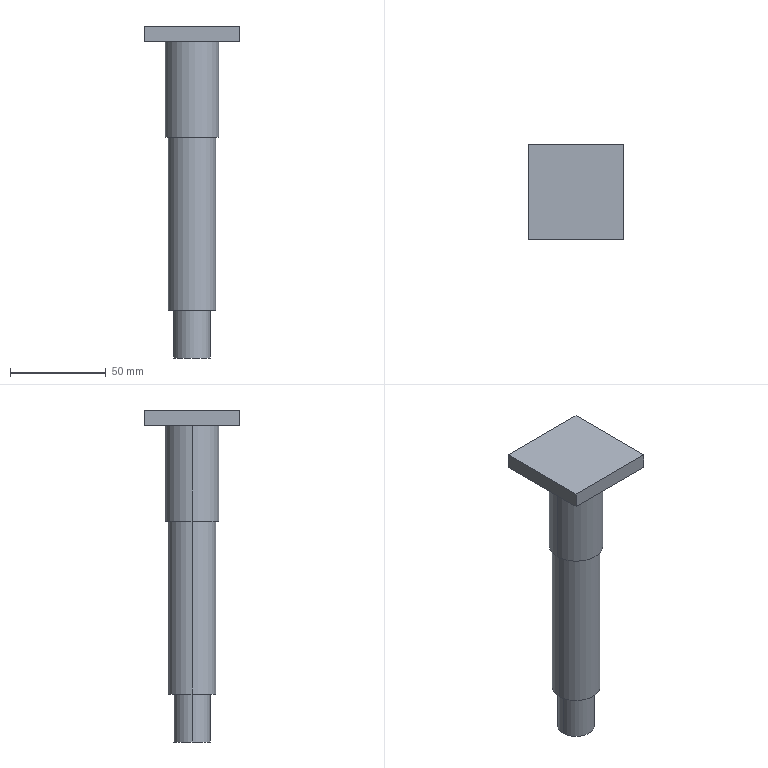Part | SolidWorks | features ICE 3, Extrusion 1 | 1 solid | 15 faces | box 50 x 50 x 173 mm | volume 102054 mm3 | plane 9 | cylinder 6 | commonest cylinder face diameters 19 x2 25 x2 28 x2
STEP:
#1=CARTESIAN_POINT('',(-9.5,0.,-25.));
#2=VERTEX_POINT('',#1);
#3=CARTESIAN_POINT('',(9.5,0.,-25.));
#4=VERTEX_POINT('',#3);
#5=CARTESIAN_POINT('',(0.,0.,-25.));
#6=DIRECTION('',(0.,0.,-1.));
#7=DIRECTION('',(-1.,0.,0.));
#8=AXIS2_PLACEMENT_3D('',#5,#6,#7);
#9=CIRCLE('',#8,9.5);
#10=EDGE_CURVE('',#2,#4,#9,.T.);
#11=ORIENTED_EDGE('',*,*,#10,.F.);
#12=CARTESIAN_POINT('',(-9.5,0.,0.));
#13=VERTEX_POINT('',#12);
#14=CARTESIAN_POINT('',(-9.5,0.,-25.));
#15=DIRECTION('',(0.,0.,1.));
#16=VECTOR('',#15,1000.);
#17=LINE('',#14,#16);
#18=EDGE_CURVE('',#2,#13,#17,.T.);
#19=ORIENTED_EDGE('',*,*,#18,.T.);
#20=CARTESIAN_POINT('',(9.5,0.,0.));
#21=VERTEX_POINT('',#20);
#22=CARTESIAN_POINT('',(0.,0.,0.));
#23=DIRECTION('',(0.,0.,-1.));
#24=DIRECTION('',(-1.,0.,0.));
#25=AXIS2_PLACEMENT_3D('',#22,#23,#24);
#26=CIRCLE('',#25,9.5);
#27=EDGE_CURVE('',#13,#21,#26,.T.);
#28=ORIENTED_EDGE('',*,*,#27,.T.);
#29=CARTESIAN_POINT('',(9.5,0.,-25.));
#30=DIRECTION('',(0.,0.,1.));
#31=VECTOR('',#30,1000.);
#32=LINE('',#29,#31);
#33=EDGE_CURVE('',#4,#21,#32,.T.);
#34=ORIENTED_EDGE('',*,*,#33,.F.);
#35=EDGE_LOOP('',(#11,#19,#28,#34));
#36=FACE_OUTER_BOUND('',#35,.T.);
#37=CARTESIAN_POINT('',(0.,0.,-25.));
#38=DIRECTION('',(0.,0.,1.));
#39=DIRECTION('',(1.,0.,0.));
#40=AXIS2_PLACEMENT_3D('',#37,#38,#39);
#41=CYLINDRICAL_SURFACE('',#40,9.5);
#42=ADVANCED_FACE('',(#36),#41,.T.);
#43=CARTESIAN_POINT('',(14.,0.,140.));
#44=VERTEX_POINT('',#43);
#45=CARTESIAN_POINT('',(-14.,0.,140.));
#46=VERTEX_POINT('',#45);
#47=CARTESIAN_POINT('',(0.,0.,140.));
#48=DIRECTION('',(0.,0.,1.));
#49=DIRECTION('',(1.,0.,0.));
#50=AXIS2_PLACEMENT_3D('',#47,#48,#49);
#51=CIRCLE('',#50,14.);
#52=EDGE_CURVE('',#44,#46,#51,.T.);
#53=ORIENTED_EDGE('',*,*,#52,.F.);
#54=CARTESIAN_POINT('',(14.,0.,90.));
#55=VERTEX_POINT('',#54);
#56=CARTESIAN_POINT('',(14.,0.,140.));
#57=DIRECTION('',(0.,0.,-1.));
#58=VECTOR('',#57,1000.);
#59=LINE('',#56,#58);
#60=EDGE_CURVE('',#44,#55,#59,.T.);
#61=ORIENTED_EDGE('',*,*,#60,.T.);
#62=CARTESIAN_POINT('',(-14.,0.,90.));
#63=VERTEX_POINT('',#62);
#64=CARTESIAN_POINT('',(0.,0.,90.));
#65=DIRECTION('',(0.,0.,1.));
#66=DIRECTION('',(1.,0.,0.));
#67=AXIS2_PLACEMENT_3D('',#64,#65,#66);
#68=CIRCLE('',#67,14.);
#69=EDGE_CURVE('',#55,#63,#68,.T.);
#70=ORIENTED_EDGE('',*,*,#69,.T.);
#71=CARTESIAN_POINT('',(-14.,0.,140.));
#72=DIRECTION('',(0.,0.,-1.));
#73=VECTOR('',#72,1000.);
#74=LINE('',#71,#73);
#75=EDGE_CURVE('',#46,#63,#74,.T.);
#76=ORIENTED_EDGE('',*,*,#75,.F.);
#77=EDGE_LOOP('',(#53,#61,#70,#76));
#78=FACE_OUTER_BOUND('',#77,.T.);
#79=CARTESIAN_POINT('',(0.,0.,140.));
#80=DIRECTION('',(0.,0.,-1.));
#81=DIRECTION('',(-1.,0.,0.));
#82=AXIS2_PLACEMENT_3D('',#79,#80,#81);
#83=CYLINDRICAL_SURFACE('',#82,14.);
#84=ADVANCED_FACE('',(#78),#83,.T.);
#85=CARTESIAN_POINT('',(12.5,0.,90.));
#86=VERTEX_POINT('',#85);
#87=CARTESIAN_POINT('',(-12.5,0.,90.));
#88=VERTEX_POINT('',#87);
#89=CARTESIAN_POINT('',(0.,0.,90.));
#90=DIRECTION('',(0.,0.,1.));
#91=DIRECTION('',(1.,0.,0.));
#92=AXIS2_PLACEMENT_3D('',#89,#90,#91);
#93=CIRCLE('',#92,12.5);
#94=EDGE_CURVE('',#86,#88,#93,.T.);
#95=ORIENTED_EDGE('',*,*,#94,.F.);
#96=CARTESIAN_POINT('',(12.5,0.,0.));
#97=VERTEX_POINT('',#96);
#98=CARTESIAN_POINT('',(12.5,0.,90.));
#99=DIRECTION('',(0.,0.,-1.));
#100=VECTOR('',#99,1000.);
#101=LINE('',#98,#100);
#102=EDGE_CURVE('',#86,#97,#101,.T.);
#103=ORIENTED_EDGE('',*,*,#102,.T.);
#104=CARTESIAN_POINT('',(-12.5,0.,0.));
#105=VERTEX_POINT('',#104);
#106=CARTESIAN_POINT('',(0.,0.,0.));
#107=DIRECTION('',(0.,0.,1.));
#108=DIRECTION('',(1.,0.,0.));
#109=AXIS2_PLACEMENT_3D('',#106,#107,#108);
#110=CIRCLE('',#109,12.5);
#111=EDGE_CURVE('',#97,#105,#110,.T.);
#112=ORIENTED_EDGE('',*,*,#111,.T.);
#113=CARTESIAN_POINT('',(-12.5,0.,90.));
#114=DIRECTION('',(0.,0.,-1.));
#115=VECTOR('',#114,1000.);
#116=LINE('',#113,#115);
#117=EDGE_CURVE('',#88,#105,#116,.T.);
#118=ORIENTED_EDGE('',*,*,#117,.F.);
#119=EDGE_LOOP('',(#95,#103,#112,#118));
#120=FACE_OUTER_BOUND('',#119,.T.);
#121=CARTESIAN_POINT('',(0.,0.,90.));
#122=DIRECTION('',(0.,0.,-1.));
#123=DIRECTION('',(-1.,0.,0.));
#124=AXIS2_PLACEMENT_3D('',#121,#122,#123);
#125=CYLINDRICAL_SURFACE('',#124,12.5);
#126=ADVANCED_FACE('',(#120),#125,.T.);
#127=ORIENTED_EDGE('',*,*,#102,.F.);
#128=CARTESIAN_POINT('',(0.,0.,90.));
#129=DIRECTION('',(0.,0.,1.));
#130=DIRECTION('',(1.,0.,0.));
#131=AXIS2_PLACEMENT_3D('',#128,#129,#130);
#132=CIRCLE('',#131,12.5);
#133=EDGE_CURVE('',#88,#86,#132,.T.);
#134=ORIENTED_EDGE('',*,*,#133,.F.);
#135=ORIENTED_EDGE('',*,*,#117,.T.);
#136=CARTESIAN_POINT('',(0.,0.,0.));
#137=DIRECTION('',(0.,0.,1.));
#138=DIRECTION('',(1.,0.,0.));
#139=AXIS2_PLACEMENT_3D('',#136,#137,#138);
#140=CIRCLE('',#139,12.5);
#141=EDGE_CURVE('',#105,#97,#140,.T.);
#142=ORIENTED_EDGE('',*,*,#141,.T.);
#143=EDGE_LOOP('',(#127,#134,#135,#142));
#144=FACE_OUTER_BOUND('',#143,.T.);
#145=CARTESIAN_POINT('',(0.,0.,90.));
#146=DIRECTION('',(0.,0.,-1.));
#147=DIRECTION('',(-1.,0.,0.));
#148=AXIS2_PLACEMENT_3D('',#145,#146,#147);
#149=CYLINDRICAL_SURFACE('',#148,12.5);
#150=ADVANCED_FACE('',(#144),#149,.T.);
#151=CARTESIAN_POINT('',(0.,0.,0.));
#152=DIRECTION('',(0.,0.,-1.));
#153=DIRECTION('',(-1.,0.,0.));
#154=AXIS2_PLACEMENT_3D('',#151,#152,#153);
#155=CIRCLE('',#154,9.5);
#156=EDGE_CURVE('',#21,#13,#155,.T.);
#157=ORIENTED_EDGE('',*,*,#156,.F.);
#158=ORIENTED_EDGE('',*,*,#27,.F.);
#159=EDGE_LOOP('',(#157,#158));
#160=FACE_BOUND('',#159,.T.);
#161=ORIENTED_EDGE('',*,*,#141,.F.);
#162=ORIENTED_EDGE('',*,*,#111,.F.);
#163=EDGE_LOOP('',(#161,#162));
#164=FACE_OUTER_BOUND('',#163,.T.);
#165=CARTESIAN_POINT('',(0.,0.,0.));
#166=DIRECTION('',(0.,0.,1.));
#167=DIRECTION('',(1.,0.,0.));
#168=AXIS2_PLACEMENT_3D('',#165,#166,#167);
#169=PLANE('',#168);
#170=ADVANCED_FACE('',(#160,#164),#169,.F.);
#171=ORIENTED_EDGE('',*,*,#60,.F.);
#172=CARTESIAN_POINT('',(0.,0.,140.));
#173=DIRECTION('',(0.,0.,1.));
#174=DIRECTION('',(1.,0.,0.));
#175=AXIS2_PLACEMENT_3D('',#172,#173,#174);
#176=CIRCLE('',#175,14.);
#177=EDGE_CURVE('',#46,#44,#176,.T.);
#178=ORIENTED_EDGE('',*,*,#177,.F.);
#179=ORIENTED_EDGE('',*,*,#75,.T.);
#180=CARTESIAN_POINT('',(0.,0.,90.));
#181=DIRECTION('',(0.,0.,1.));
#182=DIRECTION('',(1.,0.,0.));
#183=AXIS2_PLACEMENT_3D('',#180,#181,#182);
#184=CIRCLE('',#183,14.);
#185=EDGE_CURVE('',#63,#55,#184,.T.);
#186=ORIENTED_EDGE('',*,*,#185,.T.);
#187=EDGE_LOOP('',(#171,#178,#179,#186));
#188=FACE_OUTER_BOUND('',#187,.T.);
#189=CARTESIAN_POINT('',(0.,0.,140.));
#190=DIRECTION('',(0.,0.,-1.));
#191=DIRECTION('',(-1.,0.,0.));
#192=AXIS2_PLACEMENT_3D('',#189,#190,#191);
#193=CYLINDRICAL_SURFACE('',#192,14.);
#194=ADVANCED_FACE('',(#188),#193,.T.);
#195=ORIENTED_EDGE('',*,*,#133,.T.);
#196=ORIENTED_EDGE('',*,*,#94,.T.);
#197=EDGE_LOOP('',(#195,#196));
#198=FACE_BOUND('',#197,.T.);
#199=ORIENTED_EDGE('',*,*,#185,.F.);
#200=ORIENTED_EDGE('',*,*,#69,.F.);
#201=EDGE_LOOP('',(#199,#200));
#202=FACE_OUTER_BOUND('',#201,.T.);
#203=CARTESIAN_POINT('',(0.,0.,90.));
#204=DIRECTION('',(0.,0.,1.));
#205=DIRECTION('',(1.,0.,0.));
#206=AXIS2_PLACEMENT_3D('',#203,#204,#205);
#207=PLANE('',#206);
#208=ADVANCED_FACE('',(#198,#202),#207,.F.);
#209=CARTESIAN_POINT('',(25.,-25.,140.));
#210=VERTEX_POINT('',#209);
#211=CARTESIAN_POINT('',(25.,25.,140.));
#212=VERTEX_POINT('',#211);
#213=CARTESIAN_POINT('',(25.,-25.,140.));
#214=DIRECTION('',(0.,1.,0.));
#215=VECTOR('',#214,1000.);
#216=LINE('',#213,#215);
#217=EDGE_CURVE('',#210,#212,#216,.T.);
#218=ORIENTED_EDGE('',*,*,#217,.T.);
#219=CARTESIAN_POINT('',(25.,25.,148.));
#220=VERTEX_POINT('',#219);
#221=CARTESIAN_POINT('',(25.,25.,148.));
#222=DIRECTION('',(0.,0.,-1.));
#223=VECTOR('',#222,1000.);
#224=LINE('',#221,#223);
#225=EDGE_CURVE('',#220,#212,#224,.T.);
#226=ORIENTED_EDGE('',*,*,#225,.F.);
#227=CARTESIAN_POINT('',(25.,-25.,148.));
#228=VERTEX_POINT('',#227);
#229=CARTESIAN_POINT('',(25.,-25.,148.));
#230=DIRECTION('',(0.,1.,0.));
#231=VECTOR('',#230,1000.);
#232=LINE('',#229,#231);
#233=EDGE_CURVE('',#228,#220,#232,.T.);
#234=ORIENTED_EDGE('',*,*,#233,.F.);
#235=CARTESIAN_POINT('',(25.,-25.,148.));
#236=DIRECTION('',(0.,0.,-1.));
#237=VECTOR('',#236,1000.);
#238=LINE('',#235,#237);
#239=EDGE_CURVE('',#228,#210,#238,.T.);
#240=ORIENTED_EDGE('',*,*,#239,.T.);
#241=EDGE_LOOP('',(#218,#226,#234,#240));
#242=FACE_OUTER_BOUND('',#241,.T.);
#243=CARTESIAN_POINT('',(25.,-25.,148.));
#244=DIRECTION('',(-1.,0.,0.));
#245=DIRECTION('',(0.,0.,1.));
#246=AXIS2_PLACEMENT_3D('',#243,#244,#245);
#247=PLANE('',#246);
#248=ADVANCED_FACE('',(#242),#247,.F.);
#249=CARTESIAN_POINT('',(-25.,25.,140.));
#250=VERTEX_POINT('',#249);
#251=CARTESIAN_POINT('',(-25.,25.,140.));
#252=DIRECTION('',(-1.,0.,0.));
#253=VECTOR('',#252,1000.);
#254=LINE('',#251,#253);
#255=EDGE_CURVE('',#212,#250,#254,.T.);
#256=ORIENTED_EDGE('',*,*,#255,.T.);
#257=CARTESIAN_POINT('',(-25.,25.,148.));
#258=VERTEX_POINT('',#257);
#259=CARTESIAN_POINT('',(-25.,25.,148.));
#260=DIRECTION('',(0.,0.,-1.));
#261=VECTOR('',#260,1000.);
#262=LINE('',#259,#261);
#263=EDGE_CURVE('',#258,#250,#262,.T.);
#264=ORIENTED_EDGE('',*,*,#263,.F.);
#265=CARTESIAN_POINT('',(-25.,25.,148.));
#266=DIRECTION('',(-1.,0.,0.));
#267=VECTOR('',#266,1000.);
#268=LINE('',#265,#267);
#269=EDGE_CURVE('',#220,#258,#268,.T.);
#270=ORIENTED_EDGE('',*,*,#269,.F.);
#271=ORIENTED_EDGE('',*,*,#225,.T.);
#272=EDGE_LOOP('',(#256,#264,#270,#271));
#273=FACE_OUTER_BOUND('',#272,.T.);
#274=CARTESIAN_POINT('',(-25.,25.,148.));
#275=DIRECTION('',(0.,-1.,0.));
#276=DIRECTION('',(0.,0.,-1.));
#277=AXIS2_PLACEMENT_3D('',#274,#275,#276);
#278=PLANE('',#277);
#279=ADVANCED_FACE('',(#273),#278,.F.);
#280=CARTESIAN_POINT('',(-25.,-25.,140.));
#281=VERTEX_POINT('',#280);
#282=CARTESIAN_POINT('',(-25.,-25.,140.));
#283=DIRECTION('',(0.,-1.,0.));
#284=VECTOR('',#283,1000.);
#285=LINE('',#282,#284);
#286=EDGE_CURVE('',#250,#281,#285,.T.);
#287=ORIENTED_EDGE('',*,*,#286,.T.);
#288=CARTESIAN_POINT('',(-25.,-25.,148.));
#289=VERTEX_POINT('',#288);
#290=CARTESIAN_POINT('',(-25.,-25.,148.));
#291=DIRECTION('',(0.,0.,-1.));
#292=VECTOR('',#291,1000.);
#293=LINE('',#290,#292);
#294=EDGE_CURVE('',#289,#281,#293,.T.);
#295=ORIENTED_EDGE('',*,*,#294,.F.);
#296=CARTESIAN_POINT('',(-25.,-25.,148.));
#297=DIRECTION('',(0.,-1.,0.));
#298=VECTOR('',#297,1000.);
#299=LINE('',#296,#298);
#300=EDGE_CURVE('',#258,#289,#299,.T.);
#301=ORIENTED_EDGE('',*,*,#300,.F.);
#302=ORIENTED_EDGE('',*,*,#263,.T.);
#303=EDGE_LOOP('',(#287,#295,#301,#302));
#304=FACE_OUTER_BOUND('',#303,.T.);
#305=CARTESIAN_POINT('',(-25.,-25.,148.));
#306=DIRECTION('',(1.,0.,0.));
#307=DIRECTION('',(0.,0.,-1.));
#308=AXIS2_PLACEMENT_3D('',#305,#306,#307);
#309=PLANE('',#308);
#310=ADVANCED_FACE('',(#304),#309,.F.);
#311=CARTESIAN_POINT('',(-25.,-25.,140.));
#312=DIRECTION('',(1.,0.,0.));
#313=VECTOR('',#312,1000.);
#314=LINE('',#311,#313);
#315=EDGE_CURVE('',#281,#210,#314,.T.);
#316=ORIENTED_EDGE('',*,*,#315,.T.);
#317=ORIENTED_EDGE('',*,*,#239,.F.);
#318=CARTESIAN_POINT('',(-25.,-25.,148.));
#319=DIRECTION('',(1.,0.,0.));
#320=VECTOR('',#319,1000.);
#321=LINE('',#318,#320);
#322=EDGE_CURVE('',#289,#228,#321,.T.);
#323=ORIENTED_EDGE('',*,*,#322,.F.);
#324=ORIENTED_EDGE('',*,*,#294,.T.);
#325=EDGE_LOOP('',(#316,#317,#323,#324));
#326=FACE_OUTER_BOUND('',#325,.T.);
#327=CARTESIAN_POINT('',(-25.,-25.,148.));
#328=DIRECTION('',(0.,1.,0.));
#329=DIRECTION('',(0.,0.,1.));
#330=AXIS2_PLACEMENT_3D('',#327,#328,#329);
#331=PLANE('',#330);
#332=ADVANCED_FACE('',(#326),#331,.F.);
#333=ORIENTED_EDGE('',*,*,#233,.T.);
#334=ORIENTED_EDGE('',*,*,#269,.T.);
#335=ORIENTED_EDGE('',*,*,#300,.T.);
#336=ORIENTED_EDGE('',*,*,#322,.T.);
#337=EDGE_LOOP('',(#333,#334,#335,#336));
#338=FACE_OUTER_BOUND('',#337,.T.);
#339=CARTESIAN_POINT('',(0.,0.,148.));
#340=DIRECTION('',(0.,0.,-1.));
#341=DIRECTION('',(-1.,0.,0.));
#342=AXIS2_PLACEMENT_3D('',#339,#340,#341);
#343=PLANE('',#342);
#344=ADVANCED_FACE('',(#338),#343,.F.);
#345=ORIENTED_EDGE('',*,*,#177,.T.);
#346=ORIENTED_EDGE('',*,*,#52,.T.);
#347=EDGE_LOOP('',(#345,#346));
#348=FACE_BOUND('',#347,.T.);
#349=ORIENTED_EDGE('',*,*,#217,.F.);
#350=ORIENTED_EDGE('',*,*,#315,.F.);
#351=ORIENTED_EDGE('',*,*,#286,.F.);
#352=ORIENTED_EDGE('',*,*,#255,.F.);
#353=EDGE_LOOP('',(#349,#350,#351,#352));
#354=FACE_OUTER_BOUND('',#353,.T.);
#355=CARTESIAN_POINT('',(0.,0.,140.));
#356=DIRECTION('',(0.,0.,-1.));
#357=DIRECTION('',(-1.,0.,0.));
#358=AXIS2_PLACEMENT_3D('',#355,#356,#357);
#359=PLANE('',#358);
#360=ADVANCED_FACE('',(#348,#354),#359,.T.);
#361=ORIENTED_EDGE('',*,*,#18,.F.);
#362=CARTESIAN_POINT('',(0.,0.,-25.));
#363=DIRECTION('',(0.,0.,-1.));
#364=DIRECTION('',(-1.,0.,0.));
#365=AXIS2_PLACEMENT_3D('',#362,#363,#364);
#366=CIRCLE('',#365,9.5);
#367=EDGE_CURVE('',#4,#2,#366,.T.);
#368=ORIENTED_EDGE('',*,*,#367,.F.);
#369=ORIENTED_EDGE('',*,*,#33,.T.);
#370=ORIENTED_EDGE('',*,*,#156,.T.);
#371=EDGE_LOOP('',(#361,#368,#369,#370));
#372=FACE_OUTER_BOUND('',#371,.T.);
#373=CARTESIAN_POINT('',(0.,0.,-25.));
#374=DIRECTION('',(0.,0.,1.));
#375=DIRECTION('',(1.,0.,0.));
#376=AXIS2_PLACEMENT_3D('',#373,#374,#375);
#377=CYLINDRICAL_SURFACE('',#376,9.5);
#378=ADVANCED_FACE('',(#372),#377,.T.);
#379=ORIENTED_EDGE('',*,*,#367,.T.);
#380=ORIENTED_EDGE('',*,*,#10,.T.);
#381=EDGE_LOOP('',(#379,#380));
#382=FACE_OUTER_BOUND('',#381,.T.);
#383=CARTESIAN_POINT('',(0.,0.,-25.));
#384=DIRECTION('',(0.,0.,-1.));
#385=DIRECTION('',(-1.,0.,0.));
#386=AXIS2_PLACEMENT_3D('',#383,#384,#385);
#387=PLANE('',#386);
#388=ADVANCED_FACE('',(#382),#387,.T.);
#389=CLOSED_SHELL('',(#42,#84,#126,#150,#170,#194,#208,#248,#279,#310,#332,#344,#360,#378,#388));
#390=MANIFOLD_SOLID_BREP('',#389);
#391=CARTESIAN_POINT('',(0.,0.,0.));
#392=DIRECTION('',(0.,0.,1.));
#393=DIRECTION('',(1.,0.,0.));
#394=AXIS2_PLACEMENT_3D('',#391,#392,#393);
#395=(LENGTH_UNIT()NAMED_UNIT(*)SI_UNIT(.MILLI.,.METRE.));
#396=UNCERTAINTY_MEASURE_WITH_UNIT(LENGTH_MEASURE(0.00001),#395,'','');
#397=(NAMED_UNIT(*)PLANE_ANGLE_UNIT()SI_UNIT($,.RADIAN.));
#398=(NAMED_UNIT(*)SI_UNIT($,.STERADIAN.)SOLID_ANGLE_UNIT());
#399=(GEOMETRIC_REPRESENTATION_CONTEXT(3)GLOBAL_UNCERTAINTY_ASSIGNED_CONTEXT((#396))GLOBAL_UNIT_ASSIGNED_CONTEXT((#395,#397,#398))REPRESENTATION_CONTEXT('',''));
#400=ADVANCED_BREP_SHAPE_REPRESENTATION('',(#390,#394),#399);